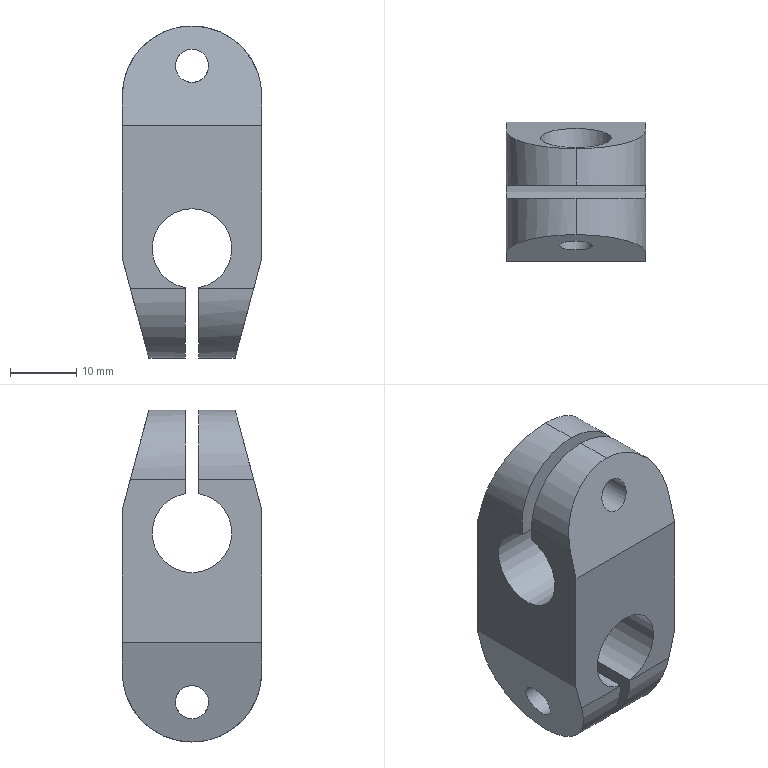Part | STEP file | 冲床-300配套压波_id470_x_t | 1 solid | 32 faces | box 21 x 21 x 50 mm | volume 11568 mm3 | cylinder 16 | plane 14 | cone 2 | commonest cylinder face diameters 21 x8 5 x2 6.8 x2 10.7 x2 12 x2
STEP:
#1=CARTESIAN_POINT('',(819.5,-112.5,-130.5));
#2=VERTEX_POINT('',#1);
#3=CARTESIAN_POINT('',(819.5,-112.5,-110.5));
#4=VERTEX_POINT('',#3);
#5=CARTESIAN_POINT('',(819.5,-112.5,-145.5));
#6=DIRECTION('',(0.,0.,1.));
#7=VECTOR('',#6,1.);
#8=LINE('',#5,#7);
#9=EDGE_CURVE('',#2,#4,#8,.T.);
#10=ORIENTED_EDGE('',*,*,#9,.F.);
#11=CARTESIAN_POINT('',(820.706,-112.5,-135.));
#12=VERTEX_POINT('',#11);
#13=CARTESIAN_POINT('',(824.657,-112.5,-149.745));
#14=DIRECTION('',(0.2588,0.,-0.9659));
#15=VECTOR('',#14,1.);
#16=LINE('',#13,#15);
#17=EDGE_CURVE('',#2,#12,#16,.T.);
#18=ORIENTED_EDGE('',*,*,#17,.T.);
#19=CARTESIAN_POINT('',(829.,-112.5,-135.));
#20=VERTEX_POINT('',#19);
#21=CARTESIAN_POINT('',(840.5,-112.5,-135.));
#22=DIRECTION('',(1.,0.,0.));
#23=VECTOR('',#22,1.);
#24=LINE('',#21,#23);
#25=EDGE_CURVE('',#12,#20,#24,.T.);
#26=ORIENTED_EDGE('',*,*,#25,.T.);
#27=CARTESIAN_POINT('',(829.,-112.5,-134.916));
#28=VERTEX_POINT('',#27);
#29=CARTESIAN_POINT('',(829.,-112.5,-152.));
#30=DIRECTION('',(0.,0.,1.));
#31=VECTOR('',#30,1.);
#32=LINE('',#29,#31);
#33=EDGE_CURVE('',#20,#28,#32,.T.);
#34=ORIENTED_EDGE('',*,*,#33,.T.);
#35=CARTESIAN_POINT('',(831.,-112.5,-134.916));
#36=VERTEX_POINT('',#35);
#37=CARTESIAN_POINT('',(830.,-112.5,-129.));
#38=DIRECTION('',(0.,-1.,0.));
#39=DIRECTION('',(0.,0.,1.));
#40=AXIS2_PLACEMENT_3D('',#37,#38,#39);
#41=CIRCLE('',#40,6.);
#42=EDGE_CURVE('',#36,#28,#41,.T.);
#43=ORIENTED_EDGE('',*,*,#42,.F.);
#44=CARTESIAN_POINT('',(831.,-112.5,-135.));
#45=VERTEX_POINT('',#44);
#46=CARTESIAN_POINT('',(831.,-112.5,-130.5));
#47=DIRECTION('',(0.,0.,-1.));
#48=VECTOR('',#47,1.);
#49=LINE('',#46,#48);
#50=EDGE_CURVE('',#36,#45,#49,.T.);
#51=ORIENTED_EDGE('',*,*,#50,.T.);
#52=CARTESIAN_POINT('',(839.294,-112.5,-135.));
#53=VERTEX_POINT('',#52);
#54=CARTESIAN_POINT('',(840.5,-112.5,-135.));
#55=DIRECTION('',(1.,0.,0.));
#56=VECTOR('',#55,1.);
#57=LINE('',#54,#56);
#58=EDGE_CURVE('',#45,#53,#57,.T.);
#59=ORIENTED_EDGE('',*,*,#58,.T.);
#60=CARTESIAN_POINT('',(840.5,-112.5,-130.5));
#61=VERTEX_POINT('',#60);
#62=CARTESIAN_POINT('',(836.75,-112.5,-144.495));
#63=DIRECTION('',(0.2588,0.,0.9659));
#64=VECTOR('',#63,1.);
#65=LINE('',#62,#64);
#66=EDGE_CURVE('',#53,#61,#65,.T.);
#67=ORIENTED_EDGE('',*,*,#66,.T.);
#68=CARTESIAN_POINT('',(840.5,-112.5,-110.5));
#69=VERTEX_POINT('',#68);
#70=CARTESIAN_POINT('',(840.5,-112.5,-145.5));
#71=DIRECTION('',(0.,0.,1.));
#72=VECTOR('',#71,1.);
#73=LINE('',#70,#72);
#74=EDGE_CURVE('',#61,#69,#73,.T.);
#75=ORIENTED_EDGE('',*,*,#74,.T.);
#76=CARTESIAN_POINT('',(840.5,-112.5,-110.5));
#77=DIRECTION('',(-1.,0.,0.));
#78=VECTOR('',#77,1.);
#79=LINE('',#76,#78);
#80=EDGE_CURVE('',#69,#4,#79,.T.);
#81=ORIENTED_EDGE('',*,*,#80,.T.);
#82=EDGE_LOOP('',(#10,#18,#26,#34,#43,#51,#59,#67,#75,#81));
#83=FACE_OUTER_BOUND('',#82,.T.);
#84=CARTESIAN_POINT('',(840.5,-112.5,-145.5));
#85=DIRECTION('',(0.,-1.,0.));
#86=DIRECTION('',(0.,0.,1.));
#87=AXIS2_PLACEMENT_3D('',#84,#85,#86);
#88=PLANE('',#87);
#89=ADVANCED_FACE('',(#83),#88,.T.);
#90=CARTESIAN_POINT('',(829.,-91.5,-135.));
#91=VERTEX_POINT('',#90);
#92=CARTESIAN_POINT('',(820.706,-91.5,-135.));
#93=VERTEX_POINT('',#92);
#94=CARTESIAN_POINT('',(840.5,-91.5,-135.));
#95=DIRECTION('',(-1.,0.,0.));
#96=VECTOR('',#95,1.);
#97=LINE('',#94,#96);
#98=EDGE_CURVE('',#91,#93,#97,.T.);
#99=ORIENTED_EDGE('',*,*,#98,.T.);
#100=CARTESIAN_POINT('',(819.5,-91.5,-130.5));
#101=VERTEX_POINT('',#100);
#102=CARTESIAN_POINT('',(812.157,-91.5,-103.095));
#103=DIRECTION('',(-0.2588,0.,0.9659));
#104=VECTOR('',#103,1.);
#105=LINE('',#102,#104);
#106=EDGE_CURVE('',#93,#101,#105,.T.);
#107=ORIENTED_EDGE('',*,*,#106,.T.);
#108=CARTESIAN_POINT('',(819.5,-91.5,-110.5));
#109=VERTEX_POINT('',#108);
#110=CARTESIAN_POINT('',(819.5,-91.5,-95.5));
#111=DIRECTION('',(0.,0.,-1.));
#112=VECTOR('',#111,1.);
#113=LINE('',#110,#112);
#114=EDGE_CURVE('',#109,#101,#113,.T.);
#115=ORIENTED_EDGE('',*,*,#114,.F.);
#116=CARTESIAN_POINT('',(840.5,-91.5,-110.5));
#117=VERTEX_POINT('',#116);
#118=CARTESIAN_POINT('',(840.5,-91.5,-110.5));
#119=DIRECTION('',(1.,0.,0.));
#120=VECTOR('',#119,1.);
#121=LINE('',#118,#120);
#122=EDGE_CURVE('',#109,#117,#121,.T.);
#123=ORIENTED_EDGE('',*,*,#122,.T.);
#124=CARTESIAN_POINT('',(840.5,-91.5,-130.5));
#125=VERTEX_POINT('',#124);
#126=CARTESIAN_POINT('',(840.5,-91.5,-95.5));
#127=DIRECTION('',(0.,0.,-1.));
#128=VECTOR('',#127,1.);
#129=LINE('',#126,#128);
#130=EDGE_CURVE('',#117,#125,#129,.T.);
#131=ORIENTED_EDGE('',*,*,#130,.T.);
#132=CARTESIAN_POINT('',(839.294,-91.5,-135.));
#133=VERTEX_POINT('',#132);
#134=CARTESIAN_POINT('',(849.25,-91.5,-97.845));
#135=DIRECTION('',(-0.2588,0.,-0.9659));
#136=VECTOR('',#135,1.);
#137=LINE('',#134,#136);
#138=EDGE_CURVE('',#125,#133,#137,.T.);
#139=ORIENTED_EDGE('',*,*,#138,.T.);
#140=CARTESIAN_POINT('',(831.,-91.5,-135.));
#141=VERTEX_POINT('',#140);
#142=CARTESIAN_POINT('',(840.5,-91.5,-135.));
#143=DIRECTION('',(-1.,0.,0.));
#144=VECTOR('',#143,1.);
#145=LINE('',#142,#144);
#146=EDGE_CURVE('',#133,#141,#145,.T.);
#147=ORIENTED_EDGE('',*,*,#146,.T.);
#148=CARTESIAN_POINT('',(831.,-91.5,-134.916));
#149=VERTEX_POINT('',#148);
#150=CARTESIAN_POINT('',(831.,-91.5,-130.5));
#151=DIRECTION('',(0.,0.,-1.));
#152=VECTOR('',#151,1.);
#153=LINE('',#150,#152);
#154=EDGE_CURVE('',#149,#141,#153,.T.);
#155=ORIENTED_EDGE('',*,*,#154,.F.);
#156=CARTESIAN_POINT('',(829.,-91.5,-134.916));
#157=VERTEX_POINT('',#156);
#158=CARTESIAN_POINT('',(830.,-91.5,-129.));
#159=DIRECTION('',(0.,-1.,0.));
#160=DIRECTION('',(0.,0.,1.));
#161=AXIS2_PLACEMENT_3D('',#158,#159,#160);
#162=CIRCLE('',#161,6.);
#163=EDGE_CURVE('',#149,#157,#162,.T.);
#164=ORIENTED_EDGE('',*,*,#163,.T.);
#165=CARTESIAN_POINT('',(829.,-91.5,-152.));
#166=DIRECTION('',(0.,0.,1.));
#167=VECTOR('',#166,1.);
#168=LINE('',#165,#167);
#169=EDGE_CURVE('',#91,#157,#168,.T.);
#170=ORIENTED_EDGE('',*,*,#169,.F.);
#171=EDGE_LOOP('',(#99,#107,#115,#123,#131,#139,#147,#155,#164,#170));
#172=FACE_OUTER_BOUND('',#171,.T.);
#173=CARTESIAN_POINT('',(840.5,-91.5,-95.5));
#174=DIRECTION('',(0.,1.,0.));
#175=DIRECTION('',(0.,0.,-1.));
#176=AXIS2_PLACEMENT_3D('',#173,#174,#175);
#177=PLANE('',#176);
#178=ADVANCED_FACE('',(#172),#177,.T.);
#179=ORIENTED_EDGE('',*,*,#114,.T.);
#180=CARTESIAN_POINT('',(819.5,445.814,-130.5));
#181=DIRECTION('',(0.,-1.,0.));
#182=VECTOR('',#181,1.);
#183=LINE('',#180,#182);
#184=EDGE_CURVE('',#101,#2,#183,.T.);
#185=ORIENTED_EDGE('',*,*,#184,.T.);
#186=ORIENTED_EDGE('',*,*,#9,.T.);
#187=CARTESIAN_POINT('',(819.5,-111.294,-106.));
#188=VERTEX_POINT('',#187);
#189=CARTESIAN_POINT('',(819.5,15.424,366.919));
#190=DIRECTION('',(0.,0.2588,0.9659));
#191=VECTOR('',#190,1.);
#192=LINE('',#189,#191);
#193=EDGE_CURVE('',#4,#188,#192,.T.);
#194=ORIENTED_EDGE('',*,*,#193,.T.);
#195=CARTESIAN_POINT('',(819.5,-103.,-106.));
#196=VERTEX_POINT('',#195);
#197=CARTESIAN_POINT('',(819.5,445.814,-106.));
#198=DIRECTION('',(0.,1.,0.));
#199=VECTOR('',#198,1.);
#200=LINE('',#197,#199);
#201=EDGE_CURVE('',#188,#196,#200,.T.);
#202=ORIENTED_EDGE('',*,*,#201,.T.);
#203=CARTESIAN_POINT('',(819.5,-103.,-108.084));
#204=VERTEX_POINT('',#203);
#205=CARTESIAN_POINT('',(819.5,-103.,-110.363));
#206=DIRECTION('',(0.,0.,1.));
#207=VECTOR('',#206,1.);
#208=LINE('',#205,#207);
#209=EDGE_CURVE('',#204,#196,#208,.T.);
#210=ORIENTED_EDGE('',*,*,#209,.F.);
#211=CARTESIAN_POINT('',(819.5,-101.,-108.084));
#212=VERTEX_POINT('',#211);
#213=CARTESIAN_POINT('',(819.5,-102.,-114.));
#214=DIRECTION('',(1.,0.,0.));
#215=DIRECTION('',(0.,0.,-1.));
#216=AXIS2_PLACEMENT_3D('',#213,#214,#215);
#217=CIRCLE('',#216,6.);
#218=EDGE_CURVE('',#204,#212,#217,.T.);
#219=ORIENTED_EDGE('',*,*,#218,.T.);
#220=CARTESIAN_POINT('',(819.5,-101.,-106.));
#221=VERTEX_POINT('',#220);
#222=CARTESIAN_POINT('',(819.5,-101.,-88.392));
#223=DIRECTION('',(0.,0.,-1.));
#224=VECTOR('',#223,1.);
#225=LINE('',#222,#224);
#226=EDGE_CURVE('',#221,#212,#225,.T.);
#227=ORIENTED_EDGE('',*,*,#226,.F.);
#228=CARTESIAN_POINT('',(819.5,-92.706,-106.));
#229=VERTEX_POINT('',#228);
#230=CARTESIAN_POINT('',(819.5,445.814,-106.));
#231=DIRECTION('',(0.,1.,0.));
#232=VECTOR('',#231,1.);
#233=LINE('',#230,#232);
#234=EDGE_CURVE('',#221,#229,#233,.T.);
#235=ORIENTED_EDGE('',*,*,#234,.T.);
#236=CARTESIAN_POINT('',(819.5,-146.031,93.012));
#237=DIRECTION('',(0.,0.2588,-0.9659));
#238=VECTOR('',#237,1.);
#239=LINE('',#236,#238);
#240=EDGE_CURVE('',#229,#109,#239,.T.);
#241=ORIENTED_EDGE('',*,*,#240,.T.);
#242=EDGE_LOOP('',(#179,#185,#186,#194,#202,#210,#219,#227,#235,#241));
#243=FACE_OUTER_BOUND('',#242,.T.);
#244=CARTESIAN_POINT('',(819.5,445.814,251.596));
#245=DIRECTION('',(-1.,0.,0.));
#246=DIRECTION('',(0.,1.,0.));
#247=AXIS2_PLACEMENT_3D('',#244,#245,#246);
#248=PLANE('',#247);
#249=ADVANCED_FACE('',(#243),#248,.T.);
#250=CARTESIAN_POINT('',(828.5,-104.5,-139.5));
#251=VERTEX_POINT('',#250);
#252=CARTESIAN_POINT('',(828.5,-102.,-139.5));
#253=DIRECTION('',(1.,0.,0.));
#254=DIRECTION('',(0.,-1.,0.));
#255=AXIS2_PLACEMENT_3D('',#252,#253,#254);
#256=CIRCLE('',#255,2.5);
#257=EDGE_CURVE('',#251,#251,#256,.T.);
#258=ORIENTED_EDGE('',*,*,#257,.T.);
#259=EDGE_LOOP('',(#258));
#260=FACE_BOUND('',#259,.T.);
#261=CARTESIAN_POINT('',(822.581,-102.,-142.));
#262=VERTEX_POINT('',#261);
#263=CARTESIAN_POINT('',(821.912,-102.,-139.5));
#264=DIRECTION('',(0.9659,0.,0.2588));
#265=DIRECTION('',(0.2588,0.,-0.9659));
#266=AXIS2_PLACEMENT_3D('',#263,#264,#265);
#267=ELLIPSE('',#266,2.588,2.5);
#268=EDGE_CURVE('',#262,#262,#267,.T.);
#269=ORIENTED_EDGE('',*,*,#268,.F.);
#270=EDGE_LOOP('',(#269));
#271=FACE_BOUND('',#270,.T.);
#272=CARTESIAN_POINT('',(793.5,-102.,-139.5));
#273=DIRECTION('',(1.,0.,0.));
#274=DIRECTION('',(0.,-1.,0.));
#275=AXIS2_PLACEMENT_3D('',#272,#273,#274);
#276=CYLINDRICAL_SURFACE('',#275,2.5);
#277=ADVANCED_FACE('',(#260,#271),#276,.F.);
#278=CARTESIAN_POINT('',(823.519,-102.,-145.5));
#279=VERTEX_POINT('',#278);
#280=CARTESIAN_POINT('',(829.,-102.,-145.5));
#281=VERTEX_POINT('',#280);
#282=CARTESIAN_POINT('',(840.5,-102.,-145.5));
#283=DIRECTION('',(1.,0.,0.));
#284=VECTOR('',#283,1.);
#285=LINE('',#282,#284);
#286=EDGE_CURVE('',#279,#281,#285,.T.);
#287=ORIENTED_EDGE('',*,*,#286,.F.);
#288=CARTESIAN_POINT('',(820.706,-102.,-135.));
#289=DIRECTION('',(0.9659,0.,0.2588));
#290=DIRECTION('',(-0.2588,0.,0.9659));
#291=AXIS2_PLACEMENT_3D('',#288,#289,#290);
#292=ELLIPSE('',#291,10.87,10.5);
#293=EDGE_CURVE('',#279,#93,#292,.T.);
#294=ORIENTED_EDGE('',*,*,#293,.T.);
#295=ORIENTED_EDGE('',*,*,#98,.F.);
#296=CARTESIAN_POINT('',(829.,-102.,-135.));
#297=DIRECTION('',(1.,0.,0.));
#298=DIRECTION('',(0.,-1.,0.));
#299=AXIS2_PLACEMENT_3D('',#296,#297,#298);
#300=CIRCLE('',#299,10.5);
#301=EDGE_CURVE('',#281,#91,#300,.T.);
#302=ORIENTED_EDGE('',*,*,#301,.F.);
#303=EDGE_LOOP('',(#287,#294,#295,#302));
#304=FACE_OUTER_BOUND('',#303,.T.);
#305=CARTESIAN_POINT('',(840.5,-102.,-135.));
#306=DIRECTION('',(-1.,0.,0.));
#307=DIRECTION('',(0.,1.,0.));
#308=AXIS2_PLACEMENT_3D('',#305,#306,#307);
#309=CYLINDRICAL_SURFACE('',#308,10.5);
#310=ADVANCED_FACE('',(#304),#309,.T.);
#311=ORIENTED_EDGE('',*,*,#25,.F.);
#312=CARTESIAN_POINT('',(820.706,-102.,-135.));
#313=DIRECTION('',(0.9659,0.,0.2588));
#314=DIRECTION('',(-0.2588,0.,0.9659));
#315=AXIS2_PLACEMENT_3D('',#312,#313,#314);
#316=ELLIPSE('',#315,10.87,10.5);
#317=EDGE_CURVE('',#12,#279,#316,.T.);
#318=ORIENTED_EDGE('',*,*,#317,.T.);
#319=ORIENTED_EDGE('',*,*,#286,.T.);
#320=CARTESIAN_POINT('',(829.,-102.,-135.));
#321=DIRECTION('',(1.,0.,0.));
#322=DIRECTION('',(0.,-1.,0.));
#323=AXIS2_PLACEMENT_3D('',#320,#321,#322);
#324=CIRCLE('',#323,10.5);
#325=EDGE_CURVE('',#20,#281,#324,.T.);
#326=ORIENTED_EDGE('',*,*,#325,.F.);
#327=EDGE_LOOP('',(#311,#318,#319,#326));
#328=FACE_OUTER_BOUND('',#327,.T.);
#329=CARTESIAN_POINT('',(840.5,-102.,-135.));
#330=DIRECTION('',(-1.,0.,0.));
#331=DIRECTION('',(0.,1.,0.));
#332=AXIS2_PLACEMENT_3D('',#329,#330,#331);
#333=CYLINDRICAL_SURFACE('',#332,10.5);
#334=ADVANCED_FACE('',(#328),#333,.T.);
#335=CARTESIAN_POINT('',(840.5,445.814,-130.5));
#336=DIRECTION('',(0.,-1.,0.));
#337=VECTOR('',#336,1.);
#338=LINE('',#335,#337);
#339=EDGE_CURVE('',#125,#61,#338,.T.);
#340=ORIENTED_EDGE('',*,*,#339,.F.);
#341=ORIENTED_EDGE('',*,*,#130,.F.);
#342=CARTESIAN_POINT('',(840.5,-92.706,-106.));
#343=VERTEX_POINT('',#342);
#344=CARTESIAN_POINT('',(840.5,-146.031,93.012));
#345=DIRECTION('',(0.,0.2588,-0.9659));
#346=VECTOR('',#345,1.);
#347=LINE('',#344,#346);
#348=EDGE_CURVE('',#343,#117,#347,.T.);
#349=ORIENTED_EDGE('',*,*,#348,.F.);
#350=CARTESIAN_POINT('',(840.5,-101.,-106.));
#351=VERTEX_POINT('',#350);
#352=CARTESIAN_POINT('',(840.5,-101.,-106.));
#353=DIRECTION('',(0.,-1.,0.));
#354=VECTOR('',#353,1.);
#355=LINE('',#352,#354);
#356=EDGE_CURVE('',#343,#351,#355,.T.);
#357=ORIENTED_EDGE('',*,*,#356,.T.);
#358=CARTESIAN_POINT('',(840.5,-101.,-108.084));
#359=VERTEX_POINT('',#358);
#360=CARTESIAN_POINT('',(840.5,-101.,-88.392));
#361=DIRECTION('',(0.,0.,-1.));
#362=VECTOR('',#361,1.);
#363=LINE('',#360,#362);
#364=EDGE_CURVE('',#351,#359,#363,.T.);
#365=ORIENTED_EDGE('',*,*,#364,.T.);
#366=CARTESIAN_POINT('',(840.5,-103.,-108.084));
#367=VERTEX_POINT('',#366);
#368=CARTESIAN_POINT('',(840.5,-102.,-114.));
#369=DIRECTION('',(1.,0.,0.));
#370=DIRECTION('',(0.,0.,-1.));
#371=AXIS2_PLACEMENT_3D('',#368,#369,#370);
#372=CIRCLE('',#371,6.);
#373=EDGE_CURVE('',#367,#359,#372,.T.);
#374=ORIENTED_EDGE('',*,*,#373,.F.);
#375=CARTESIAN_POINT('',(840.5,-103.,-106.));
#376=VERTEX_POINT('',#375);
#377=CARTESIAN_POINT('',(840.5,-103.,-110.363));
#378=DIRECTION('',(0.,0.,1.));
#379=VECTOR('',#378,1.);
#380=LINE('',#377,#379);
#381=EDGE_CURVE('',#367,#376,#380,.T.);
#382=ORIENTED_EDGE('',*,*,#381,.T.);
#383=CARTESIAN_POINT('',(840.5,-111.294,-106.));
#384=VERTEX_POINT('',#383);
#385=CARTESIAN_POINT('',(840.5,-112.5,-106.));
#386=DIRECTION('',(0.,-1.,0.));
#387=VECTOR('',#386,1.);
#388=LINE('',#385,#387);
#389=EDGE_CURVE('',#376,#384,#388,.T.);
#390=ORIENTED_EDGE('',*,*,#389,.T.);
#391=CARTESIAN_POINT('',(840.5,15.424,366.919));
#392=DIRECTION('',(0.,0.2588,0.9659));
#393=VECTOR('',#392,1.);
#394=LINE('',#391,#393);
#395=EDGE_CURVE('',#69,#384,#394,.T.);
#396=ORIENTED_EDGE('',*,*,#395,.F.);
#397=ORIENTED_EDGE('',*,*,#74,.F.);
#398=EDGE_LOOP('',(#340,#341,#349,#357,#365,#374,#382,#390,#396,#397));
#399=FACE_OUTER_BOUND('',#398,.T.);
#400=CARTESIAN_POINT('',(840.5,445.814,251.596));
#401=DIRECTION('',(-1.,0.,0.));
#402=DIRECTION('',(0.,1.,0.));
#403=AXIS2_PLACEMENT_3D('',#400,#401,#402);
#404=PLANE('',#403);
#405=ADVANCED_FACE('',(#399),#404,.F.);
#406=CARTESIAN_POINT('',(835.5,-96.65,-139.5));
#407=VERTEX_POINT('',#406);
#408=CARTESIAN_POINT('',(835.5,-102.,-139.5));
#409=DIRECTION('',(-1.,0.,0.));
#410=DIRECTION('',(0.,1.,0.));
#411=AXIS2_PLACEMENT_3D('',#408,#409,#410);
#412=CIRCLE('',#411,5.35);
#413=EDGE_CURVE('',#407,#407,#412,.T.);
#414=ORIENTED_EDGE('',*,*,#413,.T.);
#415=EDGE_LOOP('',(#414));
#416=FACE_BOUND('',#415,.T.);
#417=CARTESIAN_POINT('',(836.655,-102.,-144.85));
#418=VERTEX_POINT('',#417);
#419=CARTESIAN_POINT('',(838.088,-102.,-139.5));
#420=DIRECTION('',(0.9659,0.,-0.2588));
#421=DIRECTION('',(-0.2588,0.,-0.9659));
#422=AXIS2_PLACEMENT_3D('',#419,#420,#421);
#423=ELLIPSE('',#422,5.539,5.35);
#424=EDGE_CURVE('',#418,#418,#423,.T.);
#425=ORIENTED_EDGE('',*,*,#424,.T.);
#426=EDGE_LOOP('',(#425));
#427=FACE_BOUND('',#426,.T.);
#428=CARTESIAN_POINT('',(840.5,-102.,-139.5));
#429=DIRECTION('',(-1.,0.,0.));
#430=DIRECTION('',(0.,1.,0.));
#431=AXIS2_PLACEMENT_3D('',#428,#429,#430);
#432=CYLINDRICAL_SURFACE('',#431,5.35);
#433=ADVANCED_FACE('',(#416,#427),#432,.F.);
#434=ORIENTED_EDGE('',*,*,#146,.F.);
#435=CARTESIAN_POINT('',(836.481,-102.,-145.5));
#436=VERTEX_POINT('',#435);
#437=CARTESIAN_POINT('',(839.294,-102.,-135.));
#438=DIRECTION('',(-0.9659,0.,0.2588));
#439=DIRECTION('',(-0.2588,0.,-0.9659));
#440=AXIS2_PLACEMENT_3D('',#437,#438,#439);
#441=ELLIPSE('',#440,10.87,10.5);
#442=EDGE_CURVE('',#133,#436,#441,.T.);
#443=ORIENTED_EDGE('',*,*,#442,.T.);
#444=CARTESIAN_POINT('',(831.,-102.,-145.5));
#445=VERTEX_POINT('',#444);
#446=CARTESIAN_POINT('',(840.5,-102.,-145.5));
#447=DIRECTION('',(1.,0.,0.));
#448=VECTOR('',#447,1.);
#449=LINE('',#446,#448);
#450=EDGE_CURVE('',#445,#436,#449,.T.);
#451=ORIENTED_EDGE('',*,*,#450,.F.);
#452=CARTESIAN_POINT('',(831.,-102.,-135.));
#453=DIRECTION('',(-1.,0.,0.));
#454=DIRECTION('',(0.,1.,0.));
#455=AXIS2_PLACEMENT_3D('',#452,#453,#454);
#456=CIRCLE('',#455,10.5);
#457=EDGE_CURVE('',#141,#445,#456,.T.);
#458=ORIENTED_EDGE('',*,*,#457,.F.);
#459=EDGE_LOOP('',(#434,#443,#451,#458));
#460=FACE_OUTER_BOUND('',#459,.T.);
#461=CARTESIAN_POINT('',(840.5,-102.,-135.));
#462=DIRECTION('',(-1.,0.,0.));
#463=DIRECTION('',(0.,1.,0.));
#464=AXIS2_PLACEMENT_3D('',#461,#462,#463);
#465=CYLINDRICAL_SURFACE('',#464,10.5);
#466=ADVANCED_FACE('',(#460),#465,.T.);
#467=ORIENTED_EDGE('',*,*,#450,.T.);
#468=CARTESIAN_POINT('',(839.294,-102.,-135.));
#469=DIRECTION('',(-0.9659,0.,0.2588));
#470=DIRECTION('',(-0.2588,0.,-0.9659));
#471=AXIS2_PLACEMENT_3D('',#468,#469,#470);
#472=ELLIPSE('',#471,10.87,10.5);
#473=EDGE_CURVE('',#436,#53,#472,.T.);
#474=ORIENTED_EDGE('',*,*,#473,.T.);
#475=ORIENTED_EDGE('',*,*,#58,.F.);
#476=CARTESIAN_POINT('',(831.,-102.,-135.));
#477=DIRECTION('',(-1.,0.,0.));
#478=DIRECTION('',(0.,1.,0.));
#479=AXIS2_PLACEMENT_3D('',#476,#477,#478);
#480=CIRCLE('',#479,10.5);
#481=EDGE_CURVE('',#445,#45,#480,.T.);
#482=ORIENTED_EDGE('',*,*,#481,.F.);
#483=EDGE_LOOP('',(#467,#474,#475,#482));
#484=FACE_OUTER_BOUND('',#483,.T.);
#485=CARTESIAN_POINT('',(840.5,-102.,-135.));
#486=DIRECTION('',(-1.,0.,0.));
#487=DIRECTION('',(0.,1.,0.));
#488=AXIS2_PLACEMENT_3D('',#485,#486,#487);
#489=CYLINDRICAL_SURFACE('',#488,10.5);
#490=ADVANCED_FACE('',(#484),#489,.T.);
#491=CARTESIAN_POINT('',(830.,-108.481,-95.5));
#492=VERTEX_POINT('',#491);
#493=CARTESIAN_POINT('',(830.,-103.,-95.5));
#494=VERTEX_POINT('',#493);
#495=CARTESIAN_POINT('',(830.,-103.,-95.5));
#496=DIRECTION('',(0.,1.,0.));
#497=VECTOR('',#496,1.);
#498=LINE('',#495,#497);
#499=EDGE_CURVE('',#492,#494,#498,.T.);
#500=ORIENTED_EDGE('',*,*,#499,.F.);
#501=CARTESIAN_POINT('',(830.,-111.294,-106.));
#502=DIRECTION('',(0.,0.9659,-0.2588));
#503=DIRECTION('',(0.,-0.2588,-0.9659));
#504=AXIS2_PLACEMENT_3D('',#501,#502,#503);
#505=ELLIPSE('',#504,10.87,10.5);
#506=EDGE_CURVE('',#492,#384,#505,.T.);
#507=ORIENTED_EDGE('',*,*,#506,.T.);
#508=ORIENTED_EDGE('',*,*,#389,.F.);
#509=CARTESIAN_POINT('',(830.,-103.,-106.));
#510=DIRECTION('',(0.,1.,0.));
#511=DIRECTION('',(0.,0.,1.));
#512=AXIS2_PLACEMENT_3D('',#509,#510,#511);
#513=CIRCLE('',#512,10.5);
#514=EDGE_CURVE('',#494,#376,#513,.T.);
#515=ORIENTED_EDGE('',*,*,#514,.F.);
#516=EDGE_LOOP('',(#500,#507,#508,#515));
#517=FACE_OUTER_BOUND('',#516,.T.);
#518=CARTESIAN_POINT('',(830.,-112.5,-106.));
#519=DIRECTION('',(0.,-1.,0.));
#520=DIRECTION('',(0.,0.,1.));
#521=AXIS2_PLACEMENT_3D('',#518,#519,#520);
#522=CYLINDRICAL_SURFACE('',#521,10.5);
#523=ADVANCED_FACE('',(#517),#522,.T.);
#524=ORIENTED_EDGE('',*,*,#201,.F.);
#525=CARTESIAN_POINT('',(830.,-111.294,-106.));
#526=DIRECTION('',(0.,0.9659,-0.2588));
#527=DIRECTION('',(0.,0.2588,0.9659));
#528=AXIS2_PLACEMENT_3D('',#525,#526,#527);
#529=ELLIPSE('',#528,10.87,10.5);
#530=EDGE_CURVE('',#188,#492,#529,.T.);
#531=ORIENTED_EDGE('',*,*,#530,.T.);
#532=ORIENTED_EDGE('',*,*,#499,.T.);
#533=CARTESIAN_POINT('',(830.,-103.,-106.));
#534=DIRECTION('',(0.,1.,0.));
#535=DIRECTION('',(0.,0.,1.));
#536=AXIS2_PLACEMENT_3D('',#533,#534,#535);
#537=CIRCLE('',#536,10.5);
#538=EDGE_CURVE('',#196,#494,#537,.T.);
#539=ORIENTED_EDGE('',*,*,#538,.F.);
#540=EDGE_LOOP('',(#524,#531,#532,#539));
#541=FACE_OUTER_BOUND('',#540,.T.);
#542=CARTESIAN_POINT('',(830.,445.814,-106.));
#543=DIRECTION('',(0.,1.,0.));
#544=DIRECTION('',(0.,0.,-1.));
#545=AXIS2_PLACEMENT_3D('',#542,#543,#544);
#546=CYLINDRICAL_SURFACE('',#545,10.5);
#547=ADVANCED_FACE('',(#541),#546,.T.);
#548=CARTESIAN_POINT('',(830.,-103.5,-99.));
#549=VERTEX_POINT('',#548);
#550=CARTESIAN_POINT('',(830.,-103.5,-101.5));
#551=DIRECTION('',(0.,1.,0.));
#552=DIRECTION('',(0.,0.,1.));
#553=AXIS2_PLACEMENT_3D('',#550,#551,#552);
#554=CIRCLE('',#553,2.5);
#555=EDGE_CURVE('',#549,#549,#554,.T.);
#556=ORIENTED_EDGE('',*,*,#555,.T.);
#557=EDGE_LOOP('',(#556));
#558=FACE_BOUND('',#557,.T.);
#559=CARTESIAN_POINT('',(830.,-110.758,-104.));
#560=VERTEX_POINT('',#559);
#561=CARTESIAN_POINT('',(830.,-110.088,-101.5));
#562=DIRECTION('',(0.,0.9659,-0.2588));
#563=DIRECTION('',(0.,-0.2588,-0.9659));
#564=AXIS2_PLACEMENT_3D('',#561,#562,#563);
#565=ELLIPSE('',#564,2.588,2.5);
#566=EDGE_CURVE('',#560,#560,#565,.T.);
#567=ORIENTED_EDGE('',*,*,#566,.F.);
#568=EDGE_LOOP('',(#567));
#569=FACE_BOUND('',#568,.T.);
#570=CARTESIAN_POINT('',(830.,-127.73,-101.5));
#571=DIRECTION('',(0.,-1.,0.));
#572=DIRECTION('',(0.,0.,1.));
#573=AXIS2_PLACEMENT_3D('',#570,#571,#572);
#574=CYLINDRICAL_SURFACE('',#573,2.5);
#575=ADVANCED_FACE('',(#558,#569),#574,.F.);
#576=ORIENTED_EDGE('',*,*,#356,.F.);
#577=CARTESIAN_POINT('',(830.,-95.519,-95.5));
#578=VERTEX_POINT('',#577);
#579=CARTESIAN_POINT('',(830.,-92.706,-106.));
#580=DIRECTION('',(0.,-0.9659,-0.2588));
#581=DIRECTION('',(0.,-0.2588,0.9659));
#582=AXIS2_PLACEMENT_3D('',#579,#580,#581);
#583=ELLIPSE('',#582,10.87,10.5);
#584=EDGE_CURVE('',#343,#578,#583,.T.);
#585=ORIENTED_EDGE('',*,*,#584,.T.);
#586=CARTESIAN_POINT('',(830.,-101.,-95.5));
#587=VERTEX_POINT('',#586);
#588=CARTESIAN_POINT('',(830.,-91.5,-95.5));
#589=DIRECTION('',(0.,1.,0.));
#590=VECTOR('',#589,1.);
#591=LINE('',#588,#590);
#592=EDGE_CURVE('',#587,#578,#591,.T.);
#593=ORIENTED_EDGE('',*,*,#592,.F.);
#594=CARTESIAN_POINT('',(830.,-101.,-106.));
#595=DIRECTION('',(0.,-1.,0.));
#596=DIRECTION('',(0.,0.,-1.));
#597=AXIS2_PLACEMENT_3D('',#594,#595,#596);
#598=CIRCLE('',#597,10.5);
#599=EDGE_CURVE('',#351,#587,#598,.T.);
#600=ORIENTED_EDGE('',*,*,#599,.F.);
#601=EDGE_LOOP('',(#576,#585,#593,#600));
#602=FACE_OUTER_BOUND('',#601,.T.);
#603=CARTESIAN_POINT('',(830.,-112.5,-106.));
#604=DIRECTION('',(0.,-1.,0.));
#605=DIRECTION('',(0.,0.,1.));
#606=AXIS2_PLACEMENT_3D('',#603,#604,#605);
#607=CYLINDRICAL_SURFACE('',#606,10.5);
#608=ADVANCED_FACE('',(#602),#607,.T.);
#609=ORIENTED_EDGE('',*,*,#592,.T.);
#610=CARTESIAN_POINT('',(830.,-92.706,-106.));
#611=DIRECTION('',(0.,-0.9659,-0.2588));
#612=DIRECTION('',(0.,0.2588,-0.9659));
#613=AXIS2_PLACEMENT_3D('',#610,#611,#612);
#614=ELLIPSE('',#613,10.87,10.5);
#615=EDGE_CURVE('',#578,#229,#614,.T.);
#616=ORIENTED_EDGE('',*,*,#615,.T.);
#617=ORIENTED_EDGE('',*,*,#234,.F.);
#618=CARTESIAN_POINT('',(830.,-101.,-106.));
#619=DIRECTION('',(0.,-1.,0.));
#620=DIRECTION('',(0.,0.,-1.));
#621=AXIS2_PLACEMENT_3D('',#618,#619,#620);
#622=CIRCLE('',#621,10.5);
#623=EDGE_CURVE('',#587,#221,#622,.T.);
#624=ORIENTED_EDGE('',*,*,#623,.F.);
#625=EDGE_LOOP('',(#609,#616,#617,#624));
#626=FACE_OUTER_BOUND('',#625,.T.);
#627=CARTESIAN_POINT('',(830.,445.814,-106.));
#628=DIRECTION('',(0.,1.,0.));
#629=DIRECTION('',(0.,0.,-1.));
#630=AXIS2_PLACEMENT_3D('',#627,#628,#629);
#631=CYLINDRICAL_SURFACE('',#630,10.5);
#632=ADVANCED_FACE('',(#626),#631,.T.);
#633=CARTESIAN_POINT('',(830.,-96.5,-96.15));
#634=VERTEX_POINT('',#633);
#635=CARTESIAN_POINT('',(830.,-96.5,-101.5));
#636=DIRECTION('',(0.,1.,0.));
#637=DIRECTION('',(0.,0.,1.));
#638=AXIS2_PLACEMENT_3D('',#635,#636,#637);
#639=CIRCLE('',#638,5.35);
#640=EDGE_CURVE('',#634,#634,#639,.T.);
#641=ORIENTED_EDGE('',*,*,#640,.F.);
#642=EDGE_LOOP('',(#641));
#643=FACE_BOUND('',#642,.T.);
#644=CARTESIAN_POINT('',(830.,-95.345,-96.15));
#645=VERTEX_POINT('',#644);
#646=CARTESIAN_POINT('',(830.,-93.912,-101.5));
#647=DIRECTION('',(0.,-0.9659,-0.2588));
#648=DIRECTION('',(0.,-0.2588,0.9659));
#649=AXIS2_PLACEMENT_3D('',#646,#647,#648);
#650=ELLIPSE('',#649,5.539,5.35);
#651=EDGE_CURVE('',#645,#645,#650,.T.);
#652=ORIENTED_EDGE('',*,*,#651,.F.);
#653=EDGE_LOOP('',(#652));
#654=FACE_BOUND('',#653,.T.);
#655=CARTESIAN_POINT('',(830.,-91.5,-101.5));
#656=DIRECTION('',(0.,-1.,0.));
#657=DIRECTION('',(0.,0.,1.));
#658=AXIS2_PLACEMENT_3D('',#655,#656,#657);
#659=CYLINDRICAL_SURFACE('',#658,5.35);
#660=ADVANCED_FACE('',(#643,#654),#659,.F.);
#661=CARTESIAN_POINT('',(831.,-91.5,-134.916));
#662=DIRECTION('',(0.,1.,0.));
#663=VECTOR('',#662,1.);
#664=LINE('',#661,#663);
#665=EDGE_CURVE('',#36,#149,#664,.T.);
#666=ORIENTED_EDGE('',*,*,#665,.F.);
#667=ORIENTED_EDGE('',*,*,#42,.T.);
#668=CARTESIAN_POINT('',(829.,-91.5,-134.916));
#669=DIRECTION('',(0.,-1.,0.));
#670=VECTOR('',#669,1.);
#671=LINE('',#668,#670);
#672=EDGE_CURVE('',#157,#28,#671,.T.);
#673=ORIENTED_EDGE('',*,*,#672,.F.);
#674=ORIENTED_EDGE('',*,*,#163,.F.);
#675=EDGE_LOOP('',(#666,#667,#673,#674));
#676=FACE_OUTER_BOUND('',#675,.T.);
#677=CARTESIAN_POINT('',(830.,-91.5,-129.));
#678=DIRECTION('',(0.,-1.,0.));
#679=DIRECTION('',(0.,0.,1.));
#680=AXIS2_PLACEMENT_3D('',#677,#678,#679);
#681=CYLINDRICAL_SURFACE('',#680,6.);
#682=ADVANCED_FACE('',(#676),#681,.F.);
#683=CARTESIAN_POINT('',(830.,-101.,-104.9));
#684=VERTEX_POINT('',#683);
#685=CARTESIAN_POINT('',(830.,-101.,-101.5));
#686=DIRECTION('',(0.,1.,0.));
#687=DIRECTION('',(0.,0.,-1.));
#688=AXIS2_PLACEMENT_3D('',#685,#686,#687);
#689=CIRCLE('',#688,3.4);
#690=EDGE_CURVE('',#684,#684,#689,.T.);
#691=ORIENTED_EDGE('',*,*,#690,.T.);
#692=EDGE_LOOP('',(#691));
#693=FACE_BOUND('',#692,.T.);
#694=ORIENTED_EDGE('',*,*,#599,.T.);
#695=ORIENTED_EDGE('',*,*,#623,.T.);
#696=ORIENTED_EDGE('',*,*,#226,.T.);
#697=CARTESIAN_POINT('',(840.5,-101.,-108.084));
#698=DIRECTION('',(1.,0.,0.));
#699=VECTOR('',#698,1.);
#700=LINE('',#697,#699);
#701=EDGE_CURVE('',#212,#359,#700,.T.);
#702=ORIENTED_EDGE('',*,*,#701,.T.);
#703=ORIENTED_EDGE('',*,*,#364,.F.);
#704=EDGE_LOOP('',(#694,#695,#696,#702,#703));
#705=FACE_BOUND('',#704,.T.);
#706=CARTESIAN_POINT('',(840.5,-101.,-88.392));
#707=DIRECTION('',(0.,1.,0.));
#708=DIRECTION('',(0.,0.,-1.));
#709=AXIS2_PLACEMENT_3D('',#706,#707,#708);
#710=PLANE('',#709);
#711=ADVANCED_FACE('',(#693,#705),#710,.F.);
#712=CARTESIAN_POINT('',(840.5,-103.,-108.084));
#713=DIRECTION('',(-1.,0.,0.));
#714=VECTOR('',#713,1.);
#715=LINE('',#712,#714);
#716=EDGE_CURVE('',#367,#204,#715,.T.);
#717=ORIENTED_EDGE('',*,*,#716,.F.);
#718=ORIENTED_EDGE('',*,*,#373,.T.);
#719=ORIENTED_EDGE('',*,*,#701,.F.);
#720=ORIENTED_EDGE('',*,*,#218,.F.);
#721=EDGE_LOOP('',(#717,#718,#719,#720));
#722=FACE_OUTER_BOUND('',#721,.T.);
#723=CARTESIAN_POINT('',(840.5,-102.,-114.));
#724=DIRECTION('',(-1.,0.,0.));
#725=DIRECTION('',(0.,1.,0.));
#726=AXIS2_PLACEMENT_3D('',#723,#724,#725);
#727=CYLINDRICAL_SURFACE('',#726,6.);
#728=ADVANCED_FACE('',(#722),#727,.F.);
#729=CARTESIAN_POINT('',(830.,-103.,-98.5));
#730=VERTEX_POINT('',#729);
#731=CARTESIAN_POINT('',(830.,-103.,-101.5));
#732=DIRECTION('',(0.,-1.,0.));
#733=DIRECTION('',(0.,0.,1.));
#734=AXIS2_PLACEMENT_3D('',#731,#732,#733);
#735=CIRCLE('',#734,3.);
#736=EDGE_CURVE('',#730,#730,#735,.T.);
#737=ORIENTED_EDGE('',*,*,#736,.T.);
#738=EDGE_LOOP('',(#737));
#739=FACE_BOUND('',#738,.T.);
#740=ORIENTED_EDGE('',*,*,#209,.T.);
#741=ORIENTED_EDGE('',*,*,#538,.T.);
#742=ORIENTED_EDGE('',*,*,#514,.T.);
#743=ORIENTED_EDGE('',*,*,#381,.F.);
#744=ORIENTED_EDGE('',*,*,#716,.T.);
#745=EDGE_LOOP('',(#740,#741,#742,#743,#744));
#746=FACE_BOUND('',#745,.T.);
#747=CARTESIAN_POINT('',(840.5,-103.,-110.363));
#748=DIRECTION('',(0.,-1.,0.));
#749=DIRECTION('',(0.,0.,1.));
#750=AXIS2_PLACEMENT_3D('',#747,#748,#749);
#751=PLANE('',#750);
#752=ADVANCED_FACE('',(#739,#746),#751,.F.);
#753=CARTESIAN_POINT('',(829.,-105.,-139.5));
#754=VERTEX_POINT('',#753);
#755=CARTESIAN_POINT('',(829.,-102.,-139.5));
#756=DIRECTION('',(-1.,0.,0.));
#757=DIRECTION('',(0.,-1.,0.));
#758=AXIS2_PLACEMENT_3D('',#755,#756,#757);
#759=CIRCLE('',#758,3.);
#760=EDGE_CURVE('',#754,#754,#759,.T.);
#761=ORIENTED_EDGE('',*,*,#760,.T.);
#762=EDGE_LOOP('',(#761));
#763=FACE_BOUND('',#762,.T.);
#764=ORIENTED_EDGE('',*,*,#33,.F.);
#765=ORIENTED_EDGE('',*,*,#325,.T.);
#766=ORIENTED_EDGE('',*,*,#301,.T.);
#767=ORIENTED_EDGE('',*,*,#169,.T.);
#768=ORIENTED_EDGE('',*,*,#672,.T.);
#769=EDGE_LOOP('',(#764,#765,#766,#767,#768));
#770=FACE_BOUND('',#769,.T.);
#771=CARTESIAN_POINT('',(829.,-91.5,-152.));
#772=DIRECTION('',(1.,0.,0.));
#773=DIRECTION('',(0.,-1.,0.));
#774=AXIS2_PLACEMENT_3D('',#771,#772,#773);
#775=PLANE('',#774);
#776=ADVANCED_FACE('',(#763,#770),#775,.T.);
#777=CARTESIAN_POINT('',(831.,-98.6,-139.5));
#778=VERTEX_POINT('',#777);
#779=CARTESIAN_POINT('',(831.,-102.,-139.5));
#780=DIRECTION('',(-1.,0.,0.));
#781=DIRECTION('',(0.,1.,0.));
#782=AXIS2_PLACEMENT_3D('',#779,#780,#781);
#783=CIRCLE('',#782,3.4);
#784=EDGE_CURVE('',#778,#778,#783,.T.);
#785=ORIENTED_EDGE('',*,*,#784,.F.);
#786=EDGE_LOOP('',(#785));
#787=FACE_BOUND('',#786,.T.);
#788=ORIENTED_EDGE('',*,*,#457,.T.);
#789=ORIENTED_EDGE('',*,*,#481,.T.);
#790=ORIENTED_EDGE('',*,*,#50,.F.);
#791=ORIENTED_EDGE('',*,*,#665,.T.);
#792=ORIENTED_EDGE('',*,*,#154,.T.);
#793=EDGE_LOOP('',(#788,#789,#790,#791,#792));
#794=FACE_BOUND('',#793,.T.);
#795=CARTESIAN_POINT('',(831.,-91.5,-130.5));
#796=DIRECTION('',(-1.,0.,0.));
#797=DIRECTION('',(0.,1.,0.));
#798=AXIS2_PLACEMENT_3D('',#795,#796,#797);
#799=PLANE('',#798);
#800=ADVANCED_FACE('',(#787,#794),#799,.T.);
#801=CARTESIAN_POINT('',(835.5,-98.6,-139.5));
#802=VERTEX_POINT('',#801);
#803=CARTESIAN_POINT('',(835.5,-102.,-139.5));
#804=DIRECTION('',(1.,0.,0.));
#805=DIRECTION('',(0.,1.,0.));
#806=AXIS2_PLACEMENT_3D('',#803,#804,#805);
#807=CIRCLE('',#806,3.4);
#808=EDGE_CURVE('',#802,#802,#807,.T.);
#809=ORIENTED_EDGE('',*,*,#808,.T.);
#810=EDGE_LOOP('',(#809));
#811=FACE_BOUND('',#810,.T.);
#812=ORIENTED_EDGE('',*,*,#784,.T.);
#813=EDGE_LOOP('',(#812));
#814=FACE_BOUND('',#813,.T.);
#815=CARTESIAN_POINT('',(793.5,-102.,-139.5));
#816=DIRECTION('',(1.,0.,0.));
#817=DIRECTION('',(0.,-1.,0.));
#818=AXIS2_PLACEMENT_3D('',#815,#816,#817);
#819=CYLINDRICAL_SURFACE('',#818,3.4);
#820=ADVANCED_FACE('',(#811,#814),#819,.F.);
#821=ORIENTED_EDGE('',*,*,#413,.F.);
#822=EDGE_LOOP('',(#821));
#823=FACE_BOUND('',#822,.T.);
#824=ORIENTED_EDGE('',*,*,#808,.F.);
#825=EDGE_LOOP('',(#824));
#826=FACE_BOUND('',#825,.T.);
#827=CARTESIAN_POINT('',(835.5,-102.,-139.5));
#828=DIRECTION('',(-1.,0.,0.));
#829=DIRECTION('',(0.,1.,0.));
#830=AXIS2_PLACEMENT_3D('',#827,#828,#829);
#831=PLANE('',#830);
#832=ADVANCED_FACE('',(#823,#826),#831,.F.);
#833=CARTESIAN_POINT('',(830.,-96.5,-98.1));
#834=VERTEX_POINT('',#833);
#835=CARTESIAN_POINT('',(830.,-96.5,-101.5));
#836=DIRECTION('',(0.,1.,0.));
#837=DIRECTION('',(0.,0.,1.));
#838=AXIS2_PLACEMENT_3D('',#835,#836,#837);
#839=CIRCLE('',#838,3.4);
#840=EDGE_CURVE('',#834,#834,#839,.T.);
#841=ORIENTED_EDGE('',*,*,#840,.T.);
#842=EDGE_LOOP('',(#841));
#843=FACE_BOUND('',#842,.T.);
#844=ORIENTED_EDGE('',*,*,#690,.F.);
#845=EDGE_LOOP('',(#844));
#846=FACE_BOUND('',#845,.T.);
#847=CARTESIAN_POINT('',(830.,-127.73,-101.5));
#848=DIRECTION('',(0.,-1.,0.));
#849=DIRECTION('',(0.,0.,1.));
#850=AXIS2_PLACEMENT_3D('',#847,#848,#849);
#851=CYLINDRICAL_SURFACE('',#850,3.4);
#852=ADVANCED_FACE('',(#843,#846),#851,.F.);
#853=ORIENTED_EDGE('',*,*,#840,.F.);
#854=EDGE_LOOP('',(#853));
#855=FACE_BOUND('',#854,.T.);
#856=ORIENTED_EDGE('',*,*,#640,.T.);
#857=EDGE_LOOP('',(#856));
#858=FACE_BOUND('',#857,.T.);
#859=CARTESIAN_POINT('',(830.,-96.5,-101.5));
#860=DIRECTION('',(0.,-1.,0.));
#861=DIRECTION('',(0.,0.,1.));
#862=AXIS2_PLACEMENT_3D('',#859,#860,#861);
#863=PLANE('',#862);
#864=ADVANCED_FACE('',(#855,#858),#863,.F.);
#865=ORIENTED_EDGE('',*,*,#760,.F.);
#866=EDGE_LOOP('',(#865));
#867=FACE_BOUND('',#866,.T.);
#868=ORIENTED_EDGE('',*,*,#257,.F.);
#869=EDGE_LOOP('',(#868));
#870=FACE_BOUND('',#869,.T.);
#871=CARTESIAN_POINT('',(828.5,-102.,-139.5));
#872=DIRECTION('',(1.,0.,0.));
#873=DIRECTION('',(0.,-1.,0.));
#874=AXIS2_PLACEMENT_3D('',#871,#872,#873);
#875=CONICAL_SURFACE('',#874,2.5,45.);
#876=ADVANCED_FACE('',(#867,#870),#875,.F.);
#877=ORIENTED_EDGE('',*,*,#555,.F.);
#878=EDGE_LOOP('',(#877));
#879=FACE_BOUND('',#878,.T.);
#880=ORIENTED_EDGE('',*,*,#736,.F.);
#881=EDGE_LOOP('',(#880));
#882=FACE_BOUND('',#881,.T.);
#883=CARTESIAN_POINT('',(830.,-103.,-101.5));
#884=DIRECTION('',(0.,1.,0.));
#885=DIRECTION('',(0.,0.,-1.));
#886=AXIS2_PLACEMENT_3D('',#883,#884,#885);
#887=CONICAL_SURFACE('',#886,3.,45.);
#888=ADVANCED_FACE('',(#879,#882),#887,.F.);
#889=ORIENTED_EDGE('',*,*,#122,.F.);
#890=ORIENTED_EDGE('',*,*,#240,.F.);
#891=ORIENTED_EDGE('',*,*,#615,.F.);
#892=ORIENTED_EDGE('',*,*,#584,.F.);
#893=ORIENTED_EDGE('',*,*,#348,.T.);
#894=EDGE_LOOP('',(#889,#890,#891,#892,#893));
#895=FACE_BOUND('',#894,.T.);
#896=ORIENTED_EDGE('',*,*,#651,.T.);
#897=EDGE_LOOP('',(#896));
#898=FACE_BOUND('',#897,.T.);
#899=CARTESIAN_POINT('',(849.,-93.944,-101.378));
#900=DIRECTION('',(0.,0.9659,0.2588));
#901=DIRECTION('',(0.,0.2588,-0.9659));
#902=AXIS2_PLACEMENT_3D('',#899,#900,#901);
#903=PLANE('',#902);
#904=ADVANCED_FACE('',(#895,#898),#903,.T.);
#905=ORIENTED_EDGE('',*,*,#80,.F.);
#906=ORIENTED_EDGE('',*,*,#395,.T.);
#907=ORIENTED_EDGE('',*,*,#506,.F.);
#908=ORIENTED_EDGE('',*,*,#530,.F.);
#909=ORIENTED_EDGE('',*,*,#193,.F.);
#910=EDGE_LOOP('',(#905,#906,#907,#908,#909));
#911=FACE_BOUND('',#910,.T.);
#912=ORIENTED_EDGE('',*,*,#566,.T.);
#913=EDGE_LOOP('',(#912));
#914=FACE_BOUND('',#913,.T.);
#915=CARTESIAN_POINT('',(849.,-110.056,-101.378));
#916=DIRECTION('',(0.,-0.9659,0.2588));
#917=DIRECTION('',(0.,0.2588,0.9659));
#918=AXIS2_PLACEMENT_3D('',#915,#916,#917);
#919=PLANE('',#918);
#920=ADVANCED_FACE('',(#911,#914),#919,.T.);
#921=ORIENTED_EDGE('',*,*,#424,.F.);
#922=EDGE_LOOP('',(#921));
#923=FACE_BOUND('',#922,.T.);
#924=ORIENTED_EDGE('',*,*,#138,.F.);
#925=ORIENTED_EDGE('',*,*,#339,.T.);
#926=ORIENTED_EDGE('',*,*,#66,.F.);
#927=ORIENTED_EDGE('',*,*,#473,.F.);
#928=ORIENTED_EDGE('',*,*,#442,.F.);
#929=EDGE_LOOP('',(#924,#925,#926,#927,#928));
#930=FACE_BOUND('',#929,.T.);
#931=CARTESIAN_POINT('',(837.524,-100.,-141.608));
#932=DIRECTION('',(0.9659,0.,-0.2588));
#933=DIRECTION('',(-0.2588,0.,-0.9659));
#934=AXIS2_PLACEMENT_3D('',#931,#932,#933);
#935=PLANE('',#934);
#936=ADVANCED_FACE('',(#923,#930),#935,.T.);
#937=ORIENTED_EDGE('',*,*,#184,.F.);
#938=ORIENTED_EDGE('',*,*,#106,.F.);
#939=ORIENTED_EDGE('',*,*,#293,.F.);
#940=ORIENTED_EDGE('',*,*,#317,.F.);
#941=ORIENTED_EDGE('',*,*,#17,.F.);
#942=EDGE_LOOP('',(#937,#938,#939,#940,#941));
#943=FACE_BOUND('',#942,.T.);
#944=ORIENTED_EDGE('',*,*,#268,.T.);
#945=EDGE_LOOP('',(#944));
#946=FACE_BOUND('',#945,.T.);
#947=CARTESIAN_POINT('',(822.476,-100.,-141.608));
#948=DIRECTION('',(-0.9659,0.,-0.2588));
#949=DIRECTION('',(-0.2588,0.,0.9659));
#950=AXIS2_PLACEMENT_3D('',#947,#948,#949);
#951=PLANE('',#950);
#952=ADVANCED_FACE('',(#943,#946),#951,.T.);
#953=CLOSED_SHELL('',(#89,#178,#249,#277,#310,#334,#405,#433,#466,#490,#523,#547,#575,#608,#632,#660,#682,#711,#728,#752,#776,#800,#820,#832,#852,#864,#876,#888,#904,#920,#936,#952));
#954=MANIFOLD_SOLID_BREP('',#953);
#955=(LENGTH_UNIT()NAMED_UNIT(*)SI_UNIT(.MILLI.,.METRE.));
#956=UNCERTAINTY_MEASURE_WITH_UNIT(LENGTH_MEASURE(0.00002),#955,'','');
#957=(NAMED_UNIT(*)PLANE_ANGLE_UNIT()SI_UNIT($,.RADIAN.));
#958=PLANE_ANGLE_MEASURE_WITH_UNIT(PLANE_ANGLE_MEASURE(0.01745),#957);
#959=DIMENSIONAL_EXPONENTS(0.,0.,0.,0.,0.,0.,0.);
#960=(CONVERSION_BASED_UNIT('DEGREE',#958)NAMED_UNIT(#959)PLANE_ANGLE_UNIT());
#961=(NAMED_UNIT(*)SI_UNIT($,.STERADIAN.)SOLID_ANGLE_UNIT());
#962=(GEOMETRIC_REPRESENTATION_CONTEXT(3)GLOBAL_UNCERTAINTY_ASSIGNED_CONTEXT((#956))GLOBAL_UNIT_ASSIGNED_CONTEXT((#955,#960,#961))REPRESENTATION_CONTEXT('',''));
#963=ADVANCED_BREP_SHAPE_REPRESENTATION('',(#954),#962);